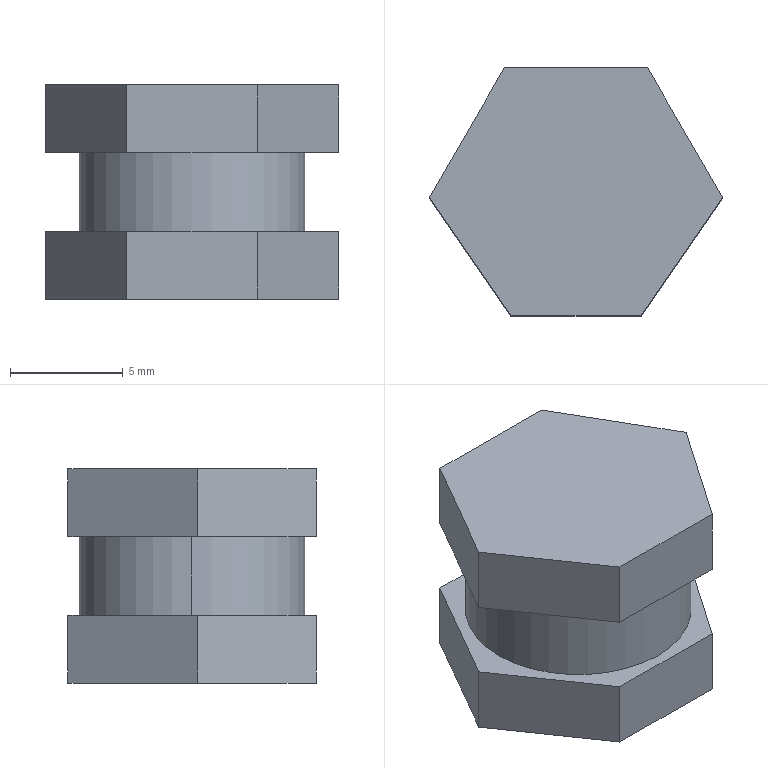Part | NX | features BREP 1 | 1 solid | 21 faces | box 13.004 x 11 x 9.5 mm | volume 595.838 mm3 | plane 17 | cylinder 4 | commonest cylinder face diameters 6.8 x2 10 x2
STEP:
#1=CARTESIAN_POINT('',(30.628,-33.241,31.812));
#2=VERTEX_POINT('',#1);
#3=CARTESIAN_POINT('',(34.243,-28.003,31.812));
#4=VERTEX_POINT('',#3);
#5=CARTESIAN_POINT('',(30.628,-33.241,31.812));
#6=DIRECTION('',(0.568,0.823,0.));
#7=VECTOR('',#6,1000.);
#8=LINE('',#5,#7);
#9=EDGE_CURVE('',#2,#4,#8,.T.);
#10=ORIENTED_EDGE('',*,*,#9,.F.);
#11=CARTESIAN_POINT('',(30.628,-33.241,28.812));
#12=VERTEX_POINT('',#11);
#13=CARTESIAN_POINT('',(30.628,-33.241,31.812));
#14=DIRECTION('',(0.,0.,-1.));
#15=VECTOR('',#14,1000.);
#16=LINE('',#13,#15);
#17=EDGE_CURVE('',#2,#12,#16,.T.);
#18=ORIENTED_EDGE('',*,*,#17,.T.);
#19=CARTESIAN_POINT('',(34.243,-28.003,28.812));
#20=VERTEX_POINT('',#19);
#21=CARTESIAN_POINT('',(34.243,-28.003,28.812));
#22=DIRECTION('',(-0.568,-0.823,0.));
#23=VECTOR('',#22,1000.);
#24=LINE('',#21,#23);
#25=EDGE_CURVE('',#20,#12,#24,.T.);
#26=ORIENTED_EDGE('',*,*,#25,.F.);
#27=CARTESIAN_POINT('',(34.243,-28.003,31.812));
#28=DIRECTION('',(0.,0.,-1.));
#29=VECTOR('',#28,1000.);
#30=LINE('',#27,#29);
#31=EDGE_CURVE('',#4,#20,#30,.T.);
#32=ORIENTED_EDGE('',*,*,#31,.F.);
#33=EDGE_LOOP('',(#10,#18,#26,#32));
#34=FACE_BOUND('',#33,.T.);
#35=CARTESIAN_POINT('',(34.243,-28.003,22.312));
#36=DIRECTION('',(0.823,-0.568,0.));
#37=DIRECTION('',(-0.568,-0.823,0.));
#38=AXIS2_PLACEMENT_3D('',#35,#36,#37);
#39=PLANE('',#38);
#40=ADVANCED_FACE('',(#34),#39,.T.);
#41=CARTESIAN_POINT('',(30.917,-22.241,31.812));
#42=VERTEX_POINT('',#41);
#43=CARTESIAN_POINT('',(34.243,-28.003,31.812));
#44=DIRECTION('',(-0.5,0.866,0.));
#45=VECTOR('',#44,1000.);
#46=LINE('',#43,#45);
#47=EDGE_CURVE('',#4,#42,#46,.T.);
#48=ORIENTED_EDGE('',*,*,#47,.F.);
#49=ORIENTED_EDGE('',*,*,#31,.T.);
#50=CARTESIAN_POINT('',(30.917,-22.241,28.812));
#51=VERTEX_POINT('',#50);
#52=CARTESIAN_POINT('',(30.917,-22.241,28.812));
#53=DIRECTION('',(0.5,-0.866,0.));
#54=VECTOR('',#53,1000.);
#55=LINE('',#52,#54);
#56=EDGE_CURVE('',#51,#20,#55,.T.);
#57=ORIENTED_EDGE('',*,*,#56,.F.);
#58=CARTESIAN_POINT('',(30.917,-22.241,31.812));
#59=DIRECTION('',(0.,0.,-1.));
#60=VECTOR('',#59,1000.);
#61=LINE('',#58,#60);
#62=EDGE_CURVE('',#42,#51,#61,.T.);
#63=ORIENTED_EDGE('',*,*,#62,.F.);
#64=EDGE_LOOP('',(#48,#49,#57,#63));
#65=FACE_BOUND('',#64,.T.);
#66=CARTESIAN_POINT('',(30.917,-22.241,22.312));
#67=DIRECTION('',(0.866,0.5,0.));
#68=DIRECTION('',(0.5,-0.866,0.));
#69=AXIS2_PLACEMENT_3D('',#66,#67,#68);
#70=PLANE('',#69);
#71=ADVANCED_FACE('',(#65),#70,.T.);
#72=CARTESIAN_POINT('',(24.566,-22.241,31.812));
#73=VERTEX_POINT('',#72);
#74=CARTESIAN_POINT('',(30.917,-22.241,31.812));
#75=DIRECTION('',(-1.,0.,0.));
#76=VECTOR('',#75,1000.);
#77=LINE('',#74,#76);
#78=EDGE_CURVE('',#42,#73,#77,.T.);
#79=ORIENTED_EDGE('',*,*,#78,.F.);
#80=ORIENTED_EDGE('',*,*,#62,.T.);
#81=CARTESIAN_POINT('',(24.566,-22.241,28.812));
#82=VERTEX_POINT('',#81);
#83=CARTESIAN_POINT('',(30.917,-22.241,28.812));
#84=DIRECTION('',(-1.,0.,0.));
#85=VECTOR('',#84,1000.);
#86=LINE('',#83,#85);
#87=EDGE_CURVE('',#51,#82,#86,.T.);
#88=ORIENTED_EDGE('',*,*,#87,.T.);
#89=CARTESIAN_POINT('',(24.566,-22.241,31.812));
#90=DIRECTION('',(0.,0.,-1.));
#91=VECTOR('',#90,1000.);
#92=LINE('',#89,#91);
#93=EDGE_CURVE('',#73,#82,#92,.T.);
#94=ORIENTED_EDGE('',*,*,#93,.F.);
#95=EDGE_LOOP('',(#79,#80,#88,#94));
#96=FACE_BOUND('',#95,.T.);
#97=CARTESIAN_POINT('',(24.566,-22.241,22.312));
#98=DIRECTION('',(0.,1.,0.));
#99=DIRECTION('',(1.,0.,0.));
#100=AXIS2_PLACEMENT_3D('',#97,#98,#99);
#101=PLANE('',#100);
#102=ADVANCED_FACE('',(#96),#101,.T.);
#103=CARTESIAN_POINT('',(21.239,-28.003,31.812));
#104=VERTEX_POINT('',#103);
#105=CARTESIAN_POINT('',(24.566,-22.241,31.812));
#106=DIRECTION('',(-0.5,-0.866,0.));
#107=VECTOR('',#106,1000.);
#108=LINE('',#105,#107);
#109=EDGE_CURVE('',#73,#104,#108,.T.);
#110=ORIENTED_EDGE('',*,*,#109,.F.);
#111=ORIENTED_EDGE('',*,*,#93,.T.);
#112=CARTESIAN_POINT('',(21.239,-28.003,28.812));
#113=VERTEX_POINT('',#112);
#114=CARTESIAN_POINT('',(21.239,-28.003,28.812));
#115=DIRECTION('',(0.5,0.866,0.));
#116=VECTOR('',#115,1000.);
#117=LINE('',#114,#116);
#118=EDGE_CURVE('',#113,#82,#117,.T.);
#119=ORIENTED_EDGE('',*,*,#118,.F.);
#120=CARTESIAN_POINT('',(21.239,-28.003,31.812));
#121=DIRECTION('',(0.,0.,-1.));
#122=VECTOR('',#121,1000.);
#123=LINE('',#120,#122);
#124=EDGE_CURVE('',#104,#113,#123,.T.);
#125=ORIENTED_EDGE('',*,*,#124,.F.);
#126=EDGE_LOOP('',(#110,#111,#119,#125));
#127=FACE_BOUND('',#126,.T.);
#128=CARTESIAN_POINT('',(21.239,-28.003,22.312));
#129=DIRECTION('',(-0.866,0.5,0.));
#130=DIRECTION('',(0.5,0.866,0.));
#131=AXIS2_PLACEMENT_3D('',#128,#129,#130);
#132=PLANE('',#131);
#133=ADVANCED_FACE('',(#127),#132,.T.);
#134=CARTESIAN_POINT('',(24.854,-33.241,31.812));
#135=VERTEX_POINT('',#134);
#136=CARTESIAN_POINT('',(21.239,-28.003,31.812));
#137=DIRECTION('',(0.568,-0.823,0.));
#138=VECTOR('',#137,1000.);
#139=LINE('',#136,#138);
#140=EDGE_CURVE('',#104,#135,#139,.T.);
#141=ORIENTED_EDGE('',*,*,#140,.F.);
#142=ORIENTED_EDGE('',*,*,#124,.T.);
#143=CARTESIAN_POINT('',(24.854,-33.241,28.812));
#144=VERTEX_POINT('',#143);
#145=CARTESIAN_POINT('',(24.854,-33.241,28.812));
#146=DIRECTION('',(-0.568,0.823,0.));
#147=VECTOR('',#146,1000.);
#148=LINE('',#145,#147);
#149=EDGE_CURVE('',#144,#113,#148,.T.);
#150=ORIENTED_EDGE('',*,*,#149,.F.);
#151=CARTESIAN_POINT('',(24.854,-33.241,31.812));
#152=DIRECTION('',(0.,0.,-1.));
#153=VECTOR('',#152,1000.);
#154=LINE('',#151,#153);
#155=EDGE_CURVE('',#135,#144,#154,.T.);
#156=ORIENTED_EDGE('',*,*,#155,.F.);
#157=EDGE_LOOP('',(#141,#142,#150,#156));
#158=FACE_BOUND('',#157,.T.);
#159=CARTESIAN_POINT('',(24.854,-33.241,22.312));
#160=DIRECTION('',(-0.823,-0.568,0.));
#161=DIRECTION('',(-0.568,0.823,0.));
#162=AXIS2_PLACEMENT_3D('',#159,#160,#161);
#163=PLANE('',#162);
#164=ADVANCED_FACE('',(#158),#163,.T.);
#165=CARTESIAN_POINT('',(24.854,-33.241,31.812));
#166=DIRECTION('',(1.,0.,0.));
#167=VECTOR('',#166,1000.);
#168=LINE('',#165,#167);
#169=EDGE_CURVE('',#135,#2,#168,.T.);
#170=ORIENTED_EDGE('',*,*,#169,.F.);
#171=ORIENTED_EDGE('',*,*,#155,.T.);
#172=CARTESIAN_POINT('',(24.854,-33.241,28.812));
#173=DIRECTION('',(1.,0.,0.));
#174=VECTOR('',#173,1000.);
#175=LINE('',#172,#174);
#176=EDGE_CURVE('',#144,#12,#175,.T.);
#177=ORIENTED_EDGE('',*,*,#176,.T.);
#178=ORIENTED_EDGE('',*,*,#17,.F.);
#179=EDGE_LOOP('',(#170,#171,#177,#178));
#180=FACE_BOUND('',#179,.T.);
#181=CARTESIAN_POINT('',(30.628,-33.241,22.312));
#182=DIRECTION('',(0.,-1.,0.));
#183=DIRECTION('',(-1.,0.,0.));
#184=AXIS2_PLACEMENT_3D('',#181,#182,#183);
#185=PLANE('',#184);
#186=ADVANCED_FACE('',(#180),#185,.T.);
#187=ORIENTED_EDGE('',*,*,#176,.F.);
#188=ORIENTED_EDGE('',*,*,#149,.T.);
#189=ORIENTED_EDGE('',*,*,#118,.T.);
#190=ORIENTED_EDGE('',*,*,#87,.F.);
#191=ORIENTED_EDGE('',*,*,#56,.T.);
#192=ORIENTED_EDGE('',*,*,#25,.T.);
#193=EDGE_LOOP('',(#187,#188,#189,#190,#191,#192));
#194=FACE_BOUND('',#193,.T.);
#195=CARTESIAN_POINT('',(22.741,-27.741,28.812));
#196=VERTEX_POINT('',#195);
#197=CARTESIAN_POINT('',(32.741,-27.741,28.812));
#198=VERTEX_POINT('',#197);
#199=CARTESIAN_POINT('',(27.741,-27.741,28.812));
#200=DIRECTION('',(0.,0.,1.));
#201=DIRECTION('',(-1.,0.,0.));
#202=AXIS2_PLACEMENT_3D('',#199,#200,#201);
#203=CIRCLE('',#202,5.);
#204=EDGE_CURVE('',#196,#198,#203,.T.);
#205=ORIENTED_EDGE('',*,*,#204,.T.);
#206=CARTESIAN_POINT('',(27.741,-27.741,28.812));
#207=DIRECTION('',(0.,0.,1.));
#208=DIRECTION('',(1.,0.,0.));
#209=AXIS2_PLACEMENT_3D('',#206,#207,#208);
#210=CIRCLE('',#209,5.);
#211=EDGE_CURVE('',#198,#196,#210,.T.);
#212=ORIENTED_EDGE('',*,*,#211,.T.);
#213=EDGE_LOOP('',(#205,#212));
#214=FACE_BOUND('',#213,.T.);
#215=CARTESIAN_POINT('',(0.,0.,28.812));
#216=DIRECTION('',(0.,0.,1.));
#217=DIRECTION('',(1.,0.,0.));
#218=AXIS2_PLACEMENT_3D('',#215,#216,#217);
#219=PLANE('',#218);
#220=ADVANCED_FACE('',(#194,#214),#219,.F.);
#221=CARTESIAN_POINT('',(22.741,-27.741,25.312));
#222=VERTEX_POINT('',#221);
#223=CARTESIAN_POINT('',(32.741,-27.741,25.312));
#224=VERTEX_POINT('',#223);
#225=CARTESIAN_POINT('',(27.741,-27.741,25.312));
#226=DIRECTION('',(0.,0.,-1.));
#227=DIRECTION('',(-1.,0.,0.));
#228=AXIS2_PLACEMENT_3D('',#225,#226,#227);
#229=CIRCLE('',#228,5.);
#230=EDGE_CURVE('',#222,#224,#229,.T.);
#231=ORIENTED_EDGE('',*,*,#230,.F.);
#232=CARTESIAN_POINT('',(22.741,-27.741,25.312));
#233=DIRECTION('',(0.,0.,1.));
#234=VECTOR('',#233,1000.);
#235=LINE('',#232,#234);
#236=EDGE_CURVE('',#222,#196,#235,.T.);
#237=ORIENTED_EDGE('',*,*,#236,.T.);
#238=ORIENTED_EDGE('',*,*,#211,.F.);
#239=CARTESIAN_POINT('',(32.741,-27.741,25.312));
#240=DIRECTION('',(0.,0.,1.));
#241=VECTOR('',#240,1000.);
#242=LINE('',#239,#241);
#243=EDGE_CURVE('',#224,#198,#242,.T.);
#244=ORIENTED_EDGE('',*,*,#243,.F.);
#245=EDGE_LOOP('',(#231,#237,#238,#244));
#246=FACE_BOUND('',#245,.T.);
#247=CARTESIAN_POINT('',(27.741,-27.741,28.812));
#248=DIRECTION('',(0.,0.,1.));
#249=DIRECTION('',(1.,0.,0.));
#250=AXIS2_PLACEMENT_3D('',#247,#248,#249);
#251=CYLINDRICAL_SURFACE('',#250,5.);
#252=ADVANCED_FACE('',(#246),#251,.T.);
#253=CARTESIAN_POINT('',(27.741,-27.741,25.312));
#254=DIRECTION('',(0.,0.,-1.));
#255=DIRECTION('',(1.,0.,0.));
#256=AXIS2_PLACEMENT_3D('',#253,#254,#255);
#257=CIRCLE('',#256,5.);
#258=EDGE_CURVE('',#224,#222,#257,.T.);
#259=ORIENTED_EDGE('',*,*,#258,.F.);
#260=ORIENTED_EDGE('',*,*,#243,.T.);
#261=ORIENTED_EDGE('',*,*,#204,.F.);
#262=ORIENTED_EDGE('',*,*,#236,.F.);
#263=EDGE_LOOP('',(#259,#260,#261,#262));
#264=FACE_BOUND('',#263,.T.);
#265=CARTESIAN_POINT('',(27.741,-27.741,28.812));
#266=DIRECTION('',(0.,0.,1.));
#267=DIRECTION('',(1.,0.,0.));
#268=AXIS2_PLACEMENT_3D('',#265,#266,#267);
#269=CYLINDRICAL_SURFACE('',#268,5.);
#270=ADVANCED_FACE('',(#264),#269,.T.);
#271=CARTESIAN_POINT('',(24.566,-22.241,25.312));
#272=VERTEX_POINT('',#271);
#273=CARTESIAN_POINT('',(21.239,-28.003,25.312));
#274=VERTEX_POINT('',#273);
#275=CARTESIAN_POINT('',(24.566,-22.241,25.312));
#276=DIRECTION('',(-0.5,-0.866,0.));
#277=VECTOR('',#276,1000.);
#278=LINE('',#275,#277);
#279=EDGE_CURVE('',#272,#274,#278,.T.);
#280=ORIENTED_EDGE('',*,*,#279,.T.);
#281=CARTESIAN_POINT('',(24.854,-33.241,25.312));
#282=VERTEX_POINT('',#281);
#283=CARTESIAN_POINT('',(21.239,-28.003,25.312));
#284=DIRECTION('',(0.568,-0.823,0.));
#285=VECTOR('',#284,1000.);
#286=LINE('',#283,#285);
#287=EDGE_CURVE('',#274,#282,#286,.T.);
#288=ORIENTED_EDGE('',*,*,#287,.T.);
#289=CARTESIAN_POINT('',(30.628,-33.241,25.312));
#290=VERTEX_POINT('',#289);
#291=CARTESIAN_POINT('',(24.854,-33.241,25.312));
#292=DIRECTION('',(1.,0.,0.));
#293=VECTOR('',#292,1000.);
#294=LINE('',#291,#293);
#295=EDGE_CURVE('',#282,#290,#294,.T.);
#296=ORIENTED_EDGE('',*,*,#295,.T.);
#297=CARTESIAN_POINT('',(34.243,-28.003,25.312));
#298=VERTEX_POINT('',#297);
#299=CARTESIAN_POINT('',(30.628,-33.241,25.312));
#300=DIRECTION('',(0.568,0.823,0.));
#301=VECTOR('',#300,1000.);
#302=LINE('',#299,#301);
#303=EDGE_CURVE('',#290,#298,#302,.T.);
#304=ORIENTED_EDGE('',*,*,#303,.T.);
#305=CARTESIAN_POINT('',(30.917,-22.241,25.312));
#306=VERTEX_POINT('',#305);
#307=CARTESIAN_POINT('',(34.243,-28.003,25.312));
#308=DIRECTION('',(-0.5,0.866,0.));
#309=VECTOR('',#308,1000.);
#310=LINE('',#307,#309);
#311=EDGE_CURVE('',#298,#306,#310,.T.);
#312=ORIENTED_EDGE('',*,*,#311,.T.);
#313=CARTESIAN_POINT('',(30.917,-22.241,25.312));
#314=DIRECTION('',(-1.,0.,0.));
#315=VECTOR('',#314,1000.);
#316=LINE('',#313,#315);
#317=EDGE_CURVE('',#306,#272,#316,.T.);
#318=ORIENTED_EDGE('',*,*,#317,.T.);
#319=EDGE_LOOP('',(#280,#288,#296,#304,#312,#318));
#320=FACE_BOUND('',#319,.T.);
#321=ORIENTED_EDGE('',*,*,#258,.T.);
#322=ORIENTED_EDGE('',*,*,#230,.T.);
#323=EDGE_LOOP('',(#321,#322));
#324=FACE_BOUND('',#323,.T.);
#325=CARTESIAN_POINT('',(0.,0.,25.312));
#326=DIRECTION('',(0.,0.,1.));
#327=DIRECTION('',(1.,0.,0.));
#328=AXIS2_PLACEMENT_3D('',#325,#326,#327);
#329=PLANE('',#328);
#330=ADVANCED_FACE('',(#320,#324),#329,.T.);
#331=CARTESIAN_POINT('',(24.566,-22.241,22.312));
#332=VERTEX_POINT('',#331);
#333=CARTESIAN_POINT('',(24.566,-22.241,25.312));
#334=DIRECTION('',(0.,0.,-1.));
#335=VECTOR('',#334,1000.);
#336=LINE('',#333,#335);
#337=EDGE_CURVE('',#272,#332,#336,.T.);
#338=ORIENTED_EDGE('',*,*,#337,.F.);
#339=ORIENTED_EDGE('',*,*,#317,.F.);
#340=CARTESIAN_POINT('',(30.917,-22.241,22.312));
#341=VERTEX_POINT('',#340);
#342=CARTESIAN_POINT('',(30.917,-22.241,25.312));
#343=DIRECTION('',(0.,0.,-1.));
#344=VECTOR('',#343,1000.);
#345=LINE('',#342,#344);
#346=EDGE_CURVE('',#306,#341,#345,.T.);
#347=ORIENTED_EDGE('',*,*,#346,.T.);
#348=CARTESIAN_POINT('',(30.917,-22.241,22.312));
#349=DIRECTION('',(-1.,0.,0.));
#350=VECTOR('',#349,1000.);
#351=LINE('',#348,#350);
#352=EDGE_CURVE('',#341,#332,#351,.T.);
#353=ORIENTED_EDGE('',*,*,#352,.T.);
#354=EDGE_LOOP('',(#338,#339,#347,#353));
#355=FACE_BOUND('',#354,.T.);
#356=CARTESIAN_POINT('',(24.566,-22.241,22.312));
#357=DIRECTION('',(0.,1.,0.));
#358=DIRECTION('',(1.,0.,0.));
#359=AXIS2_PLACEMENT_3D('',#356,#357,#358);
#360=PLANE('',#359);
#361=ADVANCED_FACE('',(#355),#360,.T.);
#362=CARTESIAN_POINT('',(24.854,-33.241,22.312));
#363=VERTEX_POINT('',#362);
#364=CARTESIAN_POINT('',(30.628,-33.241,22.312));
#365=VERTEX_POINT('',#364);
#366=CARTESIAN_POINT('',(24.854,-33.241,22.312));
#367=DIRECTION('',(1.,0.,0.));
#368=VECTOR('',#367,1000.);
#369=LINE('',#366,#368);
#370=EDGE_CURVE('',#363,#365,#369,.T.);
#371=ORIENTED_EDGE('',*,*,#370,.F.);
#372=CARTESIAN_POINT('',(21.239,-28.003,22.312));
#373=VERTEX_POINT('',#372);
#374=CARTESIAN_POINT('',(24.854,-33.241,22.312));
#375=DIRECTION('',(-0.568,0.823,0.));
#376=VECTOR('',#375,1000.);
#377=LINE('',#374,#376);
#378=EDGE_CURVE('',#363,#373,#377,.T.);
#379=ORIENTED_EDGE('',*,*,#378,.T.);
#380=CARTESIAN_POINT('',(21.239,-28.003,22.312));
#381=DIRECTION('',(0.5,0.866,0.));
#382=VECTOR('',#381,1000.);
#383=LINE('',#380,#382);
#384=EDGE_CURVE('',#373,#332,#383,.T.);
#385=ORIENTED_EDGE('',*,*,#384,.T.);
#386=ORIENTED_EDGE('',*,*,#352,.F.);
#387=CARTESIAN_POINT('',(34.243,-28.003,22.312));
#388=VERTEX_POINT('',#387);
#389=CARTESIAN_POINT('',(30.917,-22.241,22.312));
#390=DIRECTION('',(0.5,-0.866,0.));
#391=VECTOR('',#390,1000.);
#392=LINE('',#389,#391);
#393=EDGE_CURVE('',#341,#388,#392,.T.);
#394=ORIENTED_EDGE('',*,*,#393,.T.);
#395=CARTESIAN_POINT('',(34.243,-28.003,22.312));
#396=DIRECTION('',(-0.568,-0.823,0.));
#397=VECTOR('',#396,1000.);
#398=LINE('',#395,#397);
#399=EDGE_CURVE('',#388,#365,#398,.T.);
#400=ORIENTED_EDGE('',*,*,#399,.T.);
#401=EDGE_LOOP('',(#371,#379,#385,#386,#394,#400));
#402=FACE_BOUND('',#401,.T.);
#403=CARTESIAN_POINT('',(24.341,-27.741,22.312));
#404=VERTEX_POINT('',#403);
#405=CARTESIAN_POINT('',(31.141,-27.741,22.312));
#406=VERTEX_POINT('',#405);
#407=CARTESIAN_POINT('',(27.741,-27.741,22.312));
#408=DIRECTION('',(0.,0.,1.));
#409=DIRECTION('',(-1.,0.,0.));
#410=AXIS2_PLACEMENT_3D('',#407,#408,#409);
#411=CIRCLE('',#410,3.4);
#412=EDGE_CURVE('',#404,#406,#411,.T.);
#413=ORIENTED_EDGE('',*,*,#412,.T.);
#414=CARTESIAN_POINT('',(27.741,-27.741,22.312));
#415=DIRECTION('',(0.,0.,1.));
#416=DIRECTION('',(1.,0.,0.));
#417=AXIS2_PLACEMENT_3D('',#414,#415,#416);
#418=CIRCLE('',#417,3.4);
#419=EDGE_CURVE('',#406,#404,#418,.T.);
#420=ORIENTED_EDGE('',*,*,#419,.T.);
#421=EDGE_LOOP('',(#413,#420));
#422=FACE_BOUND('',#421,.T.);
#423=CARTESIAN_POINT('',(0.,0.,22.312));
#424=DIRECTION('',(0.,0.,-1.));
#425=DIRECTION('',(-1.,0.,0.));
#426=AXIS2_PLACEMENT_3D('',#423,#424,#425);
#427=PLANE('',#426);
#428=ADVANCED_FACE('',(#402,#422),#427,.T.);
#429=CARTESIAN_POINT('',(30.628,-33.241,25.312));
#430=DIRECTION('',(0.,0.,-1.));
#431=VECTOR('',#430,1000.);
#432=LINE('',#429,#431);
#433=EDGE_CURVE('',#290,#365,#432,.T.);
#434=ORIENTED_EDGE('',*,*,#433,.T.);
#435=ORIENTED_EDGE('',*,*,#399,.F.);
#436=CARTESIAN_POINT('',(34.243,-28.003,25.312));
#437=DIRECTION('',(0.,0.,-1.));
#438=VECTOR('',#437,1000.);
#439=LINE('',#436,#438);
#440=EDGE_CURVE('',#298,#388,#439,.T.);
#441=ORIENTED_EDGE('',*,*,#440,.F.);
#442=ORIENTED_EDGE('',*,*,#303,.F.);
#443=EDGE_LOOP('',(#434,#435,#441,#442));
#444=FACE_BOUND('',#443,.T.);
#445=CARTESIAN_POINT('',(34.243,-28.003,22.312));
#446=DIRECTION('',(0.823,-0.568,0.));
#447=DIRECTION('',(-0.568,-0.823,0.));
#448=AXIS2_PLACEMENT_3D('',#445,#446,#447);
#449=PLANE('',#448);
#450=ADVANCED_FACE('',(#444),#449,.T.);
#451=ORIENTED_EDGE('',*,*,#440,.T.);
#452=ORIENTED_EDGE('',*,*,#393,.F.);
#453=ORIENTED_EDGE('',*,*,#346,.F.);
#454=ORIENTED_EDGE('',*,*,#311,.F.);
#455=EDGE_LOOP('',(#451,#452,#453,#454));
#456=FACE_BOUND('',#455,.T.);
#457=CARTESIAN_POINT('',(30.917,-22.241,22.312));
#458=DIRECTION('',(0.866,0.5,0.));
#459=DIRECTION('',(0.5,-0.866,0.));
#460=AXIS2_PLACEMENT_3D('',#457,#458,#459);
#461=PLANE('',#460);
#462=ADVANCED_FACE('',(#456),#461,.T.);
#463=CARTESIAN_POINT('',(24.854,-33.241,25.312));
#464=DIRECTION('',(0.,0.,-1.));
#465=VECTOR('',#464,1000.);
#466=LINE('',#463,#465);
#467=EDGE_CURVE('',#282,#363,#466,.T.);
#468=ORIENTED_EDGE('',*,*,#467,.T.);
#469=ORIENTED_EDGE('',*,*,#370,.T.);
#470=ORIENTED_EDGE('',*,*,#433,.F.);
#471=ORIENTED_EDGE('',*,*,#295,.F.);
#472=EDGE_LOOP('',(#468,#469,#470,#471));
#473=FACE_BOUND('',#472,.T.);
#474=CARTESIAN_POINT('',(30.628,-33.241,22.312));
#475=DIRECTION('',(0.,-1.,0.));
#476=DIRECTION('',(-1.,0.,0.));
#477=AXIS2_PLACEMENT_3D('',#474,#475,#476);
#478=PLANE('',#477);
#479=ADVANCED_FACE('',(#473),#478,.T.);
#480=CARTESIAN_POINT('',(21.239,-28.003,25.312));
#481=DIRECTION('',(0.,0.,-1.));
#482=VECTOR('',#481,1000.);
#483=LINE('',#480,#482);
#484=EDGE_CURVE('',#274,#373,#483,.T.);
#485=ORIENTED_EDGE('',*,*,#484,.T.);
#486=ORIENTED_EDGE('',*,*,#378,.F.);
#487=ORIENTED_EDGE('',*,*,#467,.F.);
#488=ORIENTED_EDGE('',*,*,#287,.F.);
#489=EDGE_LOOP('',(#485,#486,#487,#488));
#490=FACE_BOUND('',#489,.T.);
#491=CARTESIAN_POINT('',(24.854,-33.241,22.312));
#492=DIRECTION('',(-0.823,-0.568,0.));
#493=DIRECTION('',(-0.568,0.823,0.));
#494=AXIS2_PLACEMENT_3D('',#491,#492,#493);
#495=PLANE('',#494);
#496=ADVANCED_FACE('',(#490),#495,.T.);
#497=ORIENTED_EDGE('',*,*,#337,.T.);
#498=ORIENTED_EDGE('',*,*,#384,.F.);
#499=ORIENTED_EDGE('',*,*,#484,.F.);
#500=ORIENTED_EDGE('',*,*,#279,.F.);
#501=EDGE_LOOP('',(#497,#498,#499,#500));
#502=FACE_BOUND('',#501,.T.);
#503=CARTESIAN_POINT('',(21.239,-28.003,22.312));
#504=DIRECTION('',(-0.866,0.5,0.));
#505=DIRECTION('',(0.5,0.866,0.));
#506=AXIS2_PLACEMENT_3D('',#503,#504,#505);
#507=PLANE('',#506);
#508=ADVANCED_FACE('',(#502),#507,.T.);
#509=ORIENTED_EDGE('',*,*,#419,.F.);
#510=CARTESIAN_POINT('',(31.141,-27.741,30.812));
#511=VERTEX_POINT('',#510);
#512=CARTESIAN_POINT('',(31.141,-27.741,30.812));
#513=DIRECTION('',(0.,0.,-1.));
#514=VECTOR('',#513,1000.);
#515=LINE('',#512,#514);
#516=EDGE_CURVE('',#511,#406,#515,.T.);
#517=ORIENTED_EDGE('',*,*,#516,.F.);
#518=CARTESIAN_POINT('',(24.341,-27.741,30.812));
#519=VERTEX_POINT('',#518);
#520=CARTESIAN_POINT('',(27.741,-27.741,30.812));
#521=DIRECTION('',(0.,0.,-1.));
#522=DIRECTION('',(-1.,0.,0.));
#523=AXIS2_PLACEMENT_3D('',#520,#521,#522);
#524=CIRCLE('',#523,3.4);
#525=EDGE_CURVE('',#519,#511,#524,.T.);
#526=ORIENTED_EDGE('',*,*,#525,.F.);
#527=CARTESIAN_POINT('',(24.341,-27.741,30.812));
#528=DIRECTION('',(0.,0.,-1.));
#529=VECTOR('',#528,1000.);
#530=LINE('',#527,#529);
#531=EDGE_CURVE('',#519,#404,#530,.T.);
#532=ORIENTED_EDGE('',*,*,#531,.T.);
#533=EDGE_LOOP('',(#509,#517,#526,#532));
#534=FACE_BOUND('',#533,.T.);
#535=CARTESIAN_POINT('',(27.741,-27.741,22.312));
#536=DIRECTION('',(0.,0.,-1.));
#537=DIRECTION('',(-1.,0.,0.));
#538=AXIS2_PLACEMENT_3D('',#535,#536,#537);
#539=CYLINDRICAL_SURFACE('',#538,3.4);
#540=ADVANCED_FACE('',(#534),#539,.F.);
#541=ORIENTED_EDGE('',*,*,#412,.F.);
#542=ORIENTED_EDGE('',*,*,#531,.F.);
#543=CARTESIAN_POINT('',(27.741,-27.741,30.812));
#544=DIRECTION('',(0.,0.,-1.));
#545=DIRECTION('',(1.,0.,0.));
#546=AXIS2_PLACEMENT_3D('',#543,#544,#545);
#547=CIRCLE('',#546,3.4);
#548=EDGE_CURVE('',#511,#519,#547,.T.);
#549=ORIENTED_EDGE('',*,*,#548,.F.);
#550=ORIENTED_EDGE('',*,*,#516,.T.);
#551=EDGE_LOOP('',(#541,#542,#549,#550));
#552=FACE_BOUND('',#551,.T.);
#553=CARTESIAN_POINT('',(27.741,-27.741,22.312));
#554=DIRECTION('',(0.,0.,-1.));
#555=DIRECTION('',(-1.,0.,0.));
#556=AXIS2_PLACEMENT_3D('',#553,#554,#555);
#557=CYLINDRICAL_SURFACE('',#556,3.4);
#558=ADVANCED_FACE('',(#552),#557,.F.);
#559=ORIENTED_EDGE('',*,*,#548,.T.);
#560=ORIENTED_EDGE('',*,*,#525,.T.);
#561=EDGE_LOOP('',(#559,#560));
#562=FACE_BOUND('',#561,.T.);
#563=CARTESIAN_POINT('',(0.,0.,30.812));
#564=DIRECTION('',(0.,0.,1.));
#565=DIRECTION('',(1.,0.,0.));
#566=AXIS2_PLACEMENT_3D('',#563,#564,#565);
#567=PLANE('',#566);
#568=ADVANCED_FACE('',(#562),#567,.F.);
#569=ORIENTED_EDGE('',*,*,#109,.T.);
#570=ORIENTED_EDGE('',*,*,#140,.T.);
#571=ORIENTED_EDGE('',*,*,#169,.T.);
#572=ORIENTED_EDGE('',*,*,#9,.T.);
#573=ORIENTED_EDGE('',*,*,#47,.T.);
#574=ORIENTED_EDGE('',*,*,#78,.T.);
#575=EDGE_LOOP('',(#569,#570,#571,#572,#573,#574));
#576=FACE_BOUND('',#575,.T.);
#577=CARTESIAN_POINT('',(0.,0.,31.812));
#578=DIRECTION('',(0.,0.,-1.));
#579=DIRECTION('',(-1.,0.,0.));
#580=AXIS2_PLACEMENT_3D('',#577,#578,#579);
#581=PLANE('',#580);
#582=ADVANCED_FACE('',(#576),#581,.F.);
#583=CLOSED_SHELL('',(#40,#71,#102,#133,#164,#186,#220,#252,#270,#330,#361,#428,#450,#462,#479,#496,#508,#540,#558,#568,#582));
#584=MANIFOLD_SOLID_BREP('',#583);
#585=(LENGTH_UNIT()NAMED_UNIT(*)SI_UNIT(.MILLI.,.METRE.));
#586=UNCERTAINTY_MEASURE_WITH_UNIT(LENGTH_MEASURE(0.00001),#585,'','');
#587=(NAMED_UNIT(*)PLANE_ANGLE_UNIT()SI_UNIT($,.RADIAN.));
#588=(NAMED_UNIT(*)SI_UNIT($,.STERADIAN.)SOLID_ANGLE_UNIT());
#589=(GEOMETRIC_REPRESENTATION_CONTEXT(3)GLOBAL_UNCERTAINTY_ASSIGNED_CONTEXT((#586))GLOBAL_UNIT_ASSIGNED_CONTEXT((#585,#587,#588))REPRESENTATION_CONTEXT('',''));
#590=ADVANCED_BREP_SHAPE_REPRESENTATION('',(#584),#589);